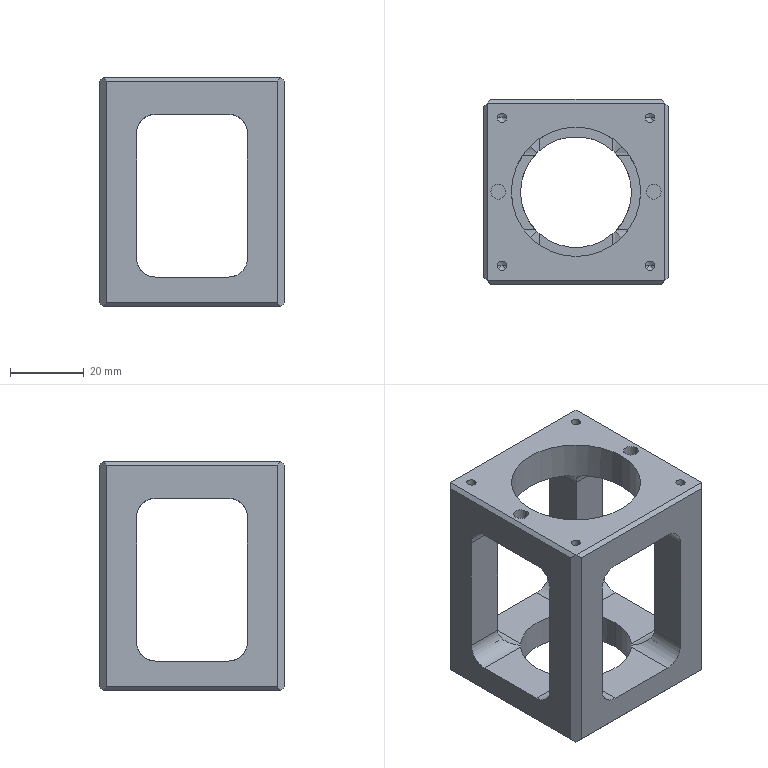Part | SolidWorks | features HoleWzd 3, ICE 3, Chamfer 2, CirPattern 1, Extrusion 1, Fillet 1, RefAxis 1 | 1 solid | 90 faces | box 50 x 50 x 62 mm | volume 46792 mm3 | cylinder 40 | plane 34 | cone 16 | commonest cylinder face diameters 10 x16 2.5 x8 3.3 x8 4 x4 30 x2 35 x2